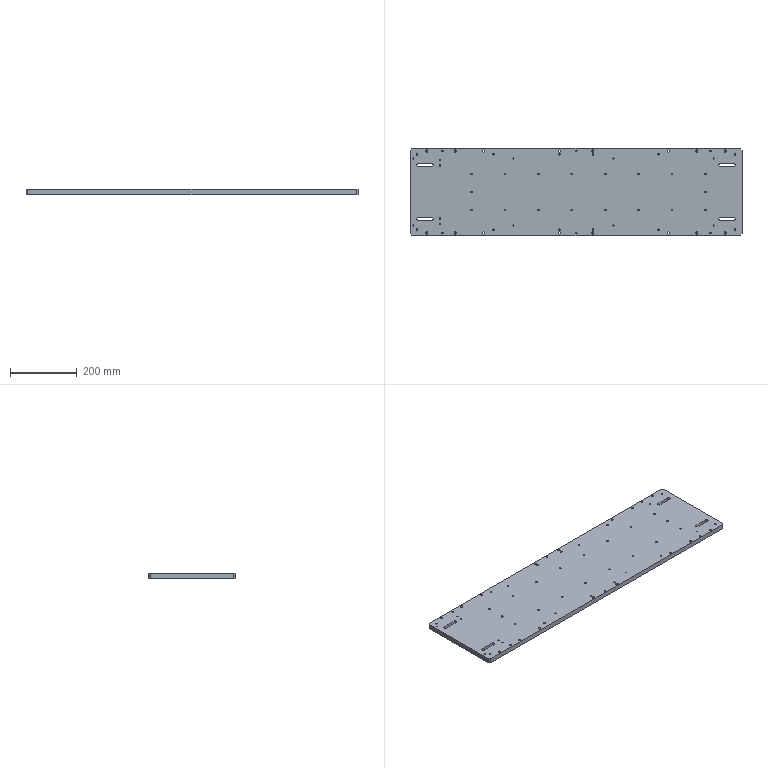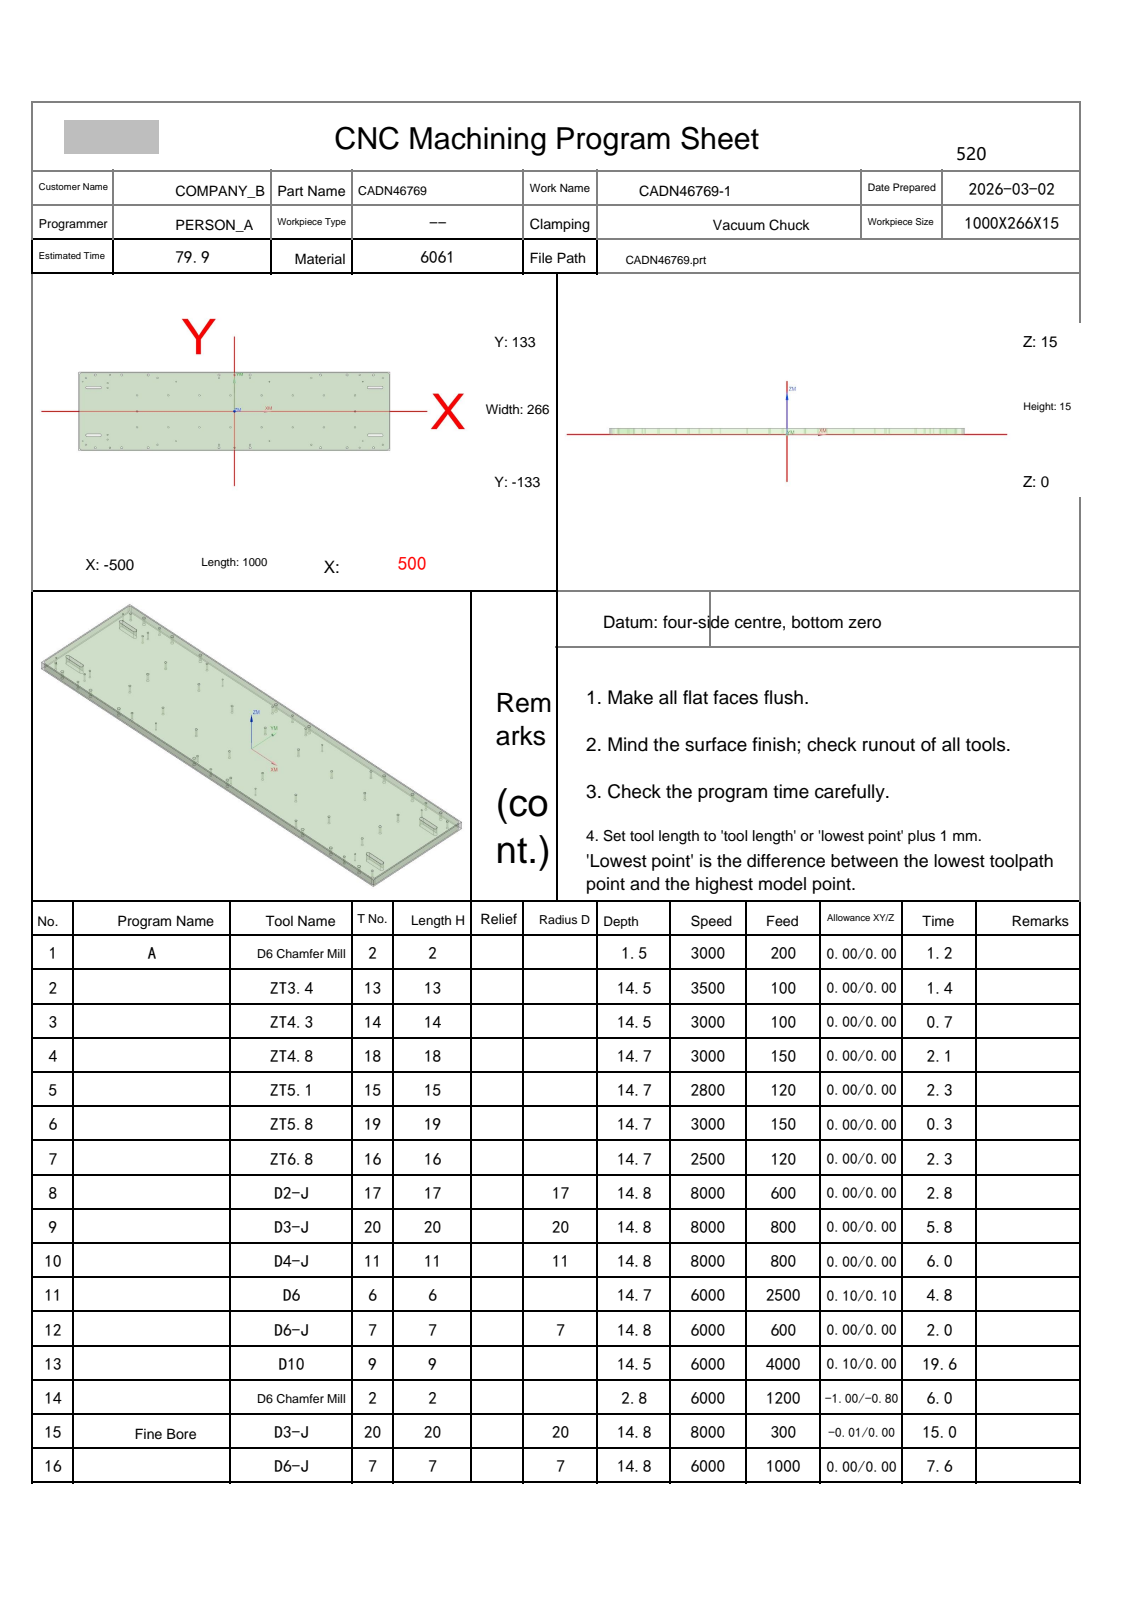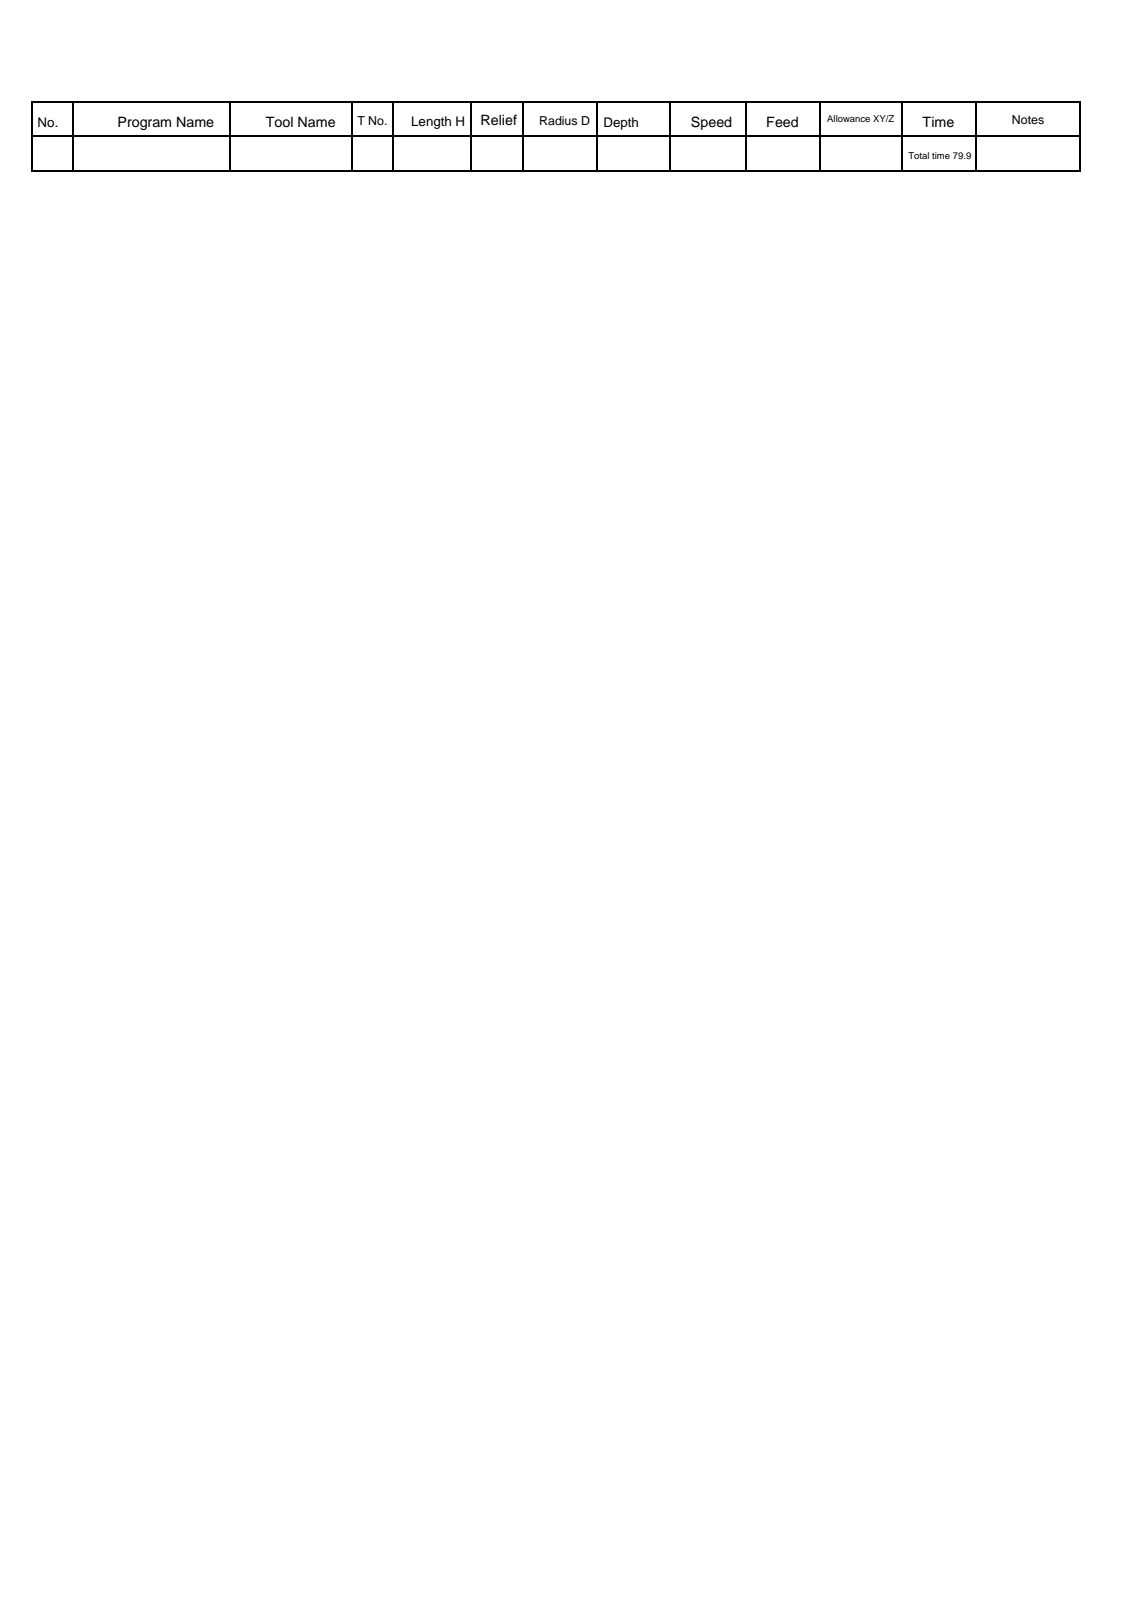NC program | NX | posted by the shop | part box 995 x 261 x 15 mm
Lines 235 to 1015 of 14350:
N8 T17 M06
(D2-J  D=2. R=0. H=17 ce=0.00 di=0.00)
G00 G90 G54 X-486.9 Y-100.369 M03 S8000
G43 H17 Z45.
M08
Z15.5
G01 X-486.943 Y-100.227 Z15.492 F600.
X-487.061 Y-100.061 Z15.482
X-487.227 Y-99.943 Z15.471
X-487.421 Y-99.884 Z15.46
X-487.579 Z15.452
X-487.765 Y-99.939 Z15.442
X-487.926 Y-100.049 Z15.432
X-488.045 Y-100.203 Z15.421
X-488.11 Y-100.386 Z15.411
X-488.116 Y-100.579 Z15.401
X-488.057 Y-100.773 Z15.39
X-487.939 Y-100.939 Z15.38
X-487.773 Y-101.057 Z15.369
X-487.579 Y-101.116 Z15.358
X-487.421 Z15.35
X-487.227 Y-101.057 Z15.34
X-487.061 Y-100.939 Z15.329
X-486.943 Y-100.773 Z15.318
X-486.884 Y-100.579 Z15.308
Y-100.421 Z15.299
X-486.943 Y-100.227 Z15.289
X-487.061 Y-100.061 Z15.278
X-487.227 Y-99.943 Z15.267
X-487.421 Y-99.884 Z15.257
X-487.579 Z15.248
X-487.765 Y-99.939 Z15.238
X-487.926 Y-100.049 Z15.228
X-488.045 Y-100.203 Z15.218
X-488.11 Y-100.386 Z15.208
X-488.116 Y-100.579 Z15.198
X-488.057 Y-100.773 Z15.187
X-487.939 Y-100.939 Z15.176
X-487.773 Y-101.057 Z15.166
X-487.579 Y-101.116 Z15.155
X-487.421 Z15.147
X-487.227 Y-101.057 Z15.136
X-487.061 Y-100.939 Z15.125
X-486.943 Y-100.773 Z15.115
X-486.884 Y-100.579 Z15.104
Y-100.421 Z15.096
X-486.943 Y-100.227 Z15.085
X-487.061 Y-100.061 Z15.074
X-487.227 Y-99.943 Z15.064
X-487.421 Y-99.884 Z15.053
X-487.579 Z15.045
X-487.765 Y-99.939 Z15.035
X-487.926 Y-100.049 Z15.025
X-488.045 Y-100.203 Z15.014
X-488.11 Y-100.386 Z15.004
X-488.115 Y-100.465 Z15.
G41 D17
X-488.15 Y-100.5
G03 X-487.5 Y-101.15 Z14.914 I.65 J0.0
X-486.85 Y-100.5 Z14.828 I0.0 J.65
X-487.5 Y-99.85 Z14.742 I-.65 J0.0
X-488.15 Y-100.5 Z14.656 I0.0 J-.65
X-487.5 Y-101.15 Z14.57 I.65 J0.0
X-486.85 Y-100.5 Z14.484 I0.0 J.65
X-487.5 Y-99.85 Z14.398 I-.65 J0.0
X-488.15 Y-100.5 Z14.312 I0.0 J-.65
X-487.5 Y-101.15 Z14.226 I.65 J0.0
X-486.85 Y-100.5 Z14.14 I0.0 J.65
X-487.5 Y-99.85 Z14.053 I-.65 J0.0
X-488.15 Y-100.5 Z13.967 I0.0 J-.65
X-487.5 Y-101.15 Z13.881 I.65 J0.0
X-486.85 Y-100.5 Z13.795 I0.0 J.65
X-487.5 Y-99.85 Z13.709 I-.65 J0.0
X-488.15 Y-100.5 Z13.623 I0.0 J-.65
X-487.5 Y-101.15 Z13.537 I.65 J0.0
X-486.85 Y-100.5 Z13.451 I0.0 J.65
X-487.5 Y-99.85 Z13.365 I-.65 J0.0
X-488.15 Y-100.5 Z13.279 I0.0 J-.65
X-487.5 Y-101.15 Z13.193 I.65 J0.0
X-486.85 Y-100.5 Z13.107 I0.0 J.65
X-487.5 Y-99.85 Z13.021 I-.65 J0.0
X-488.15 Y-100.5 Z12.935 I0.0 J-.65
X-487.5 Y-101.15 Z12.849 I.65 J0.0
X-486.85 Y-100.5 Z12.763 I0.0 J.65
X-487.5 Y-99.85 Z12.677 I-.65 J0.0
X-488.15 Y-100.5 Z12.591 I0.0 J-.65
X-487.5 Y-101.15 Z12.505 I.65 J0.0
X-486.85 Y-100.5 Z12.419 I0.0 J.65
X-487.5 Y-99.85 Z12.333 I-.65 J0.0
X-488.15 Y-100.5 Z12.247 I0.0 J-.65
X-487.5 Y-101.15 Z12.16 I.65 J0.0
X-486.85 Y-100.5 Z12.074 I0.0 J.65
X-487.5 Y-99.85 Z11.988 I-.65 J0.0
X-488.15 Y-100.5 Z11.902 I0.0 J-.65
X-487.5 Y-101.15 Z11.816 I.65 J0.0
X-486.85 Y-100.5 Z11.73 I0.0 J.65
X-487.5 Y-99.85 Z11.644 I-.65 J0.0
X-488.15 Y-100.5 Z11.558 I0.0 J-.65
X-487.5 Y-101.15 Z11.472 I.65 J0.0
X-486.85 Y-100.5 Z11.386 I0.0 J.65
X-487.5 Y-99.85 Z11.3 I-.65 J0.0
X-488.15 Y-100.5 Z11.214 I0.0 J-.65
X-487.5 Y-101.15 Z11.128 I.65 J0.0
X-486.85 Y-100.5 Z11.042 I0.0 J.65
X-487.5 Y-99.85 Z10.956 I-.65 J0.0
X-488.15 Y-100.5 Z10.87 I0.0 J-.65
X-487.5 Y-101.15 Z10.784 I.65 J0.0
X-486.85 Y-100.5 Z10.698 I0.0 J.65
X-487.5 Y-99.85 Z10.612 I-.65 J0.0
X-488.15 Y-100.5 Z10.526 I0.0 J-.65
X-487.5 Y-101.15 Z10.44 I.65 J0.0
X-486.85 Y-100.5 Z10.353 I0.0 J.65
X-487.5 Y-99.85 Z10.267 I-.65 J0.0
X-488.15 Y-100.5 Z10.181 I0.0 J-.65
X-487.5 Y-101.15 Z10.095 I.65 J0.0
X-486.85 Y-100.5 Z10.009 I0.0 J.65
X-487.5 Y-99.85 Z9.923 I-.65 J0.0
X-488.15 Y-100.5 Z9.837 I0.0 J-.65
X-487.5 Y-101.15 Z9.751 I.65 J0.0
X-486.85 Y-100.5 Z9.665 I0.0 J.65
X-487.5 Y-99.85 Z9.579 I-.65 J0.0
X-488.15 Y-100.5 Z9.493 I0.0 J-.65
X-487.5 Y-101.15 Z9.407 I.65 J0.0
X-486.85 Y-100.5 Z9.321 I0.0 J.65
X-487.5 Y-99.85 Z9.235 I-.65 J0.0
X-488.15 Y-100.5 Z9.149 I0.0 J-.65
X-487.5 Y-101.15 Z9.063 I.65 J0.0
X-486.85 Y-100.5 Z8.977 I0.0 J.65
X-487.5 Y-99.85 Z8.891 I-.65 J0.0
X-488.15 Y-100.5 Z8.805 I0.0 J-.65
X-487.5 Y-101.15 Z8.719 I.65 J0.0
X-486.85 Y-100.5 Z8.633 I0.0 J.65
X-487.5 Y-99.85 Z8.547 I-.65 J0.0
X-488.15 Y-100.5 Z8.46 I0.0 J-.65
X-487.5 Y-101.15 Z8.374 I.65 J0.0
X-486.85 Y-100.5 Z8.288 I0.0 J.65
X-487.5 Y-99.85 Z8.202 I-.65 J0.0
X-488.15 Y-100.5 Z8.116 I0.0 J-.65
X-487.5 Y-101.15 Z8.03 I.65 J0.0
X-486.85 Y-100.5 Z7.944 I0.0 J.65
X-487.5 Y-99.85 Z7.858 I-.65 J0.0
X-488.15 Y-100.5 Z7.772 I0.0 J-.65
X-487.5 Y-101.15 Z7.686 I.65 J0.0
X-486.85 Y-100.5 Z7.6 I0.0 J.65
X-487.5 Y-99.85 Z7.514 I-.65 J0.0
X-488.15 Y-100.5 Z7.428 I0.0 J-.65
X-487.5 Y-101.15 Z7.342 I.65 J0.0
X-486.85 Y-100.5 Z7.256 I0.0 J.65
X-487.5 Y-99.85 Z7.17 I-.65 J0.0
X-488.15 Y-100.5 Z7.084 I0.0 J-.65
X-487.5 Y-101.15 Z6.998 I.65 J0.0
X-486.85 Y-100.5 Z6.912 I0.0 J.65
X-487.5 Y-99.85 Z6.826 I-.65 J0.0
X-488.15 Y-100.5 Z6.74 I0.0 J-.65
X-487.5 Y-101.15 Z6.653 I.65 J0.0
X-486.85 Y-100.5 Z6.567 I0.0 J.65
X-487.5 Y-99.85 Z6.481 I-.65 J0.0
X-488.15 Y-100.5 Z6.395 I0.0 J-.65
X-487.5 Y-101.15 Z6.309 I.65 J0.0
X-486.85 Y-100.5 Z6.223 I0.0 J.65
X-487.5 Y-99.85 Z6.137 I-.65 J0.0
X-488.15 Y-100.5 Z6.051 I0.0 J-.65
X-487.5 Y-101.15 Z5.965 I.65 J0.0
X-486.85 Y-100.5 Z5.879 I0.0 J.65
X-487.5 Y-99.85 Z5.793 I-.65 J0.0
X-488.15 Y-100.5 Z5.707 I0.0 J-.65
X-487.5 Y-101.15 Z5.621 I.65 J0.0
X-486.85 Y-100.5 Z5.535 I0.0 J.65
X-487.5 Y-99.85 Z5.449 I-.65 J0.0
X-488.15 Y-100.5 Z5.363 I0.0 J-.65
X-487.5 Y-101.15 Z5.277 I.65 J0.0
X-486.85 Y-100.5 Z5.191 I0.0 J.65
X-487.5 Y-99.85 Z5.105 I-.65 J0.0
X-488.15 Y-100.5 Z5.019 I0.0 J-.65
X-487.5 Y-101.15 Z4.933 I.65 J0.0
X-486.85 Y-100.5 Z4.847 I0.0 J.65
X-487.5 Y-99.85 Z4.76 I-.65 J0.0
X-488.15 Y-100.5 Z4.674 I0.0 J-.65
X-487.5 Y-101.15 Z4.588 I.65 J0.0
X-486.85 Y-100.5 Z4.502 I0.0 J.65
X-487.5 Y-99.85 Z4.416 I-.65 J0.0
X-488.15 Y-100.5 Z4.33 I0.0 J-.65
X-487.5 Y-101.15 Z4.244 I.65 J0.0
X-486.85 Y-100.5 Z4.158 I0.0 J.65
X-487.5 Y-99.85 Z4.072 I-.65 J0.0
X-488.15 Y-100.5 Z3.986 I0.0 J-.65
X-487.5 Y-101.15 Z3.9 I.65 J0.0
X-486.85 Y-100.5 Z3.814 I0.0 J.65
X-487.5 Y-99.85 Z3.728 I-.65 J0.0
X-488.15 Y-100.5 Z3.642 I0.0 J-.65
X-487.5 Y-101.15 Z3.556 I.65 J0.0
X-486.85 Y-100.5 Z3.47 I0.0 J.65
X-487.5 Y-99.85 Z3.384 I-.65 J0.0
X-488.15 Y-100.5 Z3.298 I0.0 J-.65
X-487.5 Y-101.15 Z3.212 I.65 J0.0
X-486.85 Y-100.5 Z3.126 I0.0 J.65
X-487.5 Y-99.85 Z3.04 I-.65 J0.0
X-488.15 Y-100.5 Z2.953 I0.0 J-.65
X-487.5 Y-101.15 Z2.867 I.65 J0.0
X-486.85 Y-100.5 Z2.781 I0.0 J.65
X-487.5 Y-99.85 Z2.695 I-.65 J0.0
X-488.15 Y-100.5 Z2.609 I0.0 J-.65
X-487.5 Y-101.15 Z2.523 I.65 J0.0
X-486.85 Y-100.5 Z2.437 I0.0 J.65
X-487.5 Y-99.85 Z2.351 I-.65 J0.0
X-488.15 Y-100.5 Z2.265 I0.0 J-.65
X-487.5 Y-101.15 Z2.179 I.65 J0.0
X-486.85 Y-100.5 Z2.093 I0.0 J.65
X-487.5 Y-99.85 Z2.007 I-.65 J0.0
X-488.15 Y-100.5 Z1.921 I0.0 J-.65
X-487.5 Y-101.15 Z1.835 I.65 J0.0
X-486.85 Y-100.5 Z1.749 I0.0 J.65
X-487.5 Y-99.85 Z1.663 I-.65 J0.0
X-488.15 Y-100.5 Z1.577 I0.0 J-.65
X-487.5 Y-101.15 Z1.491 I.65 J0.0
X-486.85 Y-100.5 Z1.405 I0.0 J.65
X-487.5 Y-99.85 Z1.319 I-.65 J0.0
X-488.15 Y-100.5 Z1.233 I0.0 J-.65
X-487.5 Y-101.15 Z1.147 I.65 J0.0
X-486.85 Y-100.5 Z1.06 I0.0 J.65
X-487.5 Y-99.85 Z.974 I-.65 J0.0
X-488.15 Y-100.5 Z.888 I0.0 J-.65
X-487.5 Y-101.15 Z.802 I.65 J0.0
X-486.85 Y-100.5 Z.716 I0.0 J.65
X-487.5 Y-99.85 Z.63 I-.65 J0.0
X-488.15 Y-100.5 Z.544 I0.0 J-.65
X-487.5 Y-101.15 Z.458 I.65 J0.0
X-486.85 Y-100.5 Z.372 I0.0 J.65
X-487.5 Y-99.85 Z.286 I-.65 J0.0
X-488.15 Y-100.5 Z.2 I0.0 J-.65
X-487.5 Y-101.15 I.65 J0.0
X-486.85 Y-100.5 I0.0 J.65
X-487.5 Y-99.85 I-.65 J0.0
X-488.15 Y-100.5 I0.0 J-.65
X-488.031 Y-100.875 I.65 J0.0
G01 X-488.013 Y-100.896
X-487.985 Y-100.901
X-487.961 Y-100.887
G40 X-487.92 Y-100.858
Z1.2
G00 Z45.
X-486.9 Y100.631
Z15.5
G01 X-486.943 Y100.773 Z15.492
X-487.061 Y100.939 Z15.482
X-487.227 Y101.057 Z15.471
X-487.421 Y101.116 Z15.46
X-487.579 Z15.452
X-487.765 Y101.061 Z15.442
X-487.926 Y100.951 Z15.432
X-488.045 Y100.797 Z15.421
X-488.11 Y100.614 Z15.411
X-488.116 Y100.421 Z15.401
X-488.057 Y100.227 Z15.39
X-487.939 Y100.061 Z15.38
X-487.773 Y99.943 Z15.369
X-487.579 Y99.884 Z15.358
X-487.421 Z15.35
X-487.227 Y99.943 Z15.34
X-487.061 Y100.061 Z15.329
X-486.943 Y100.227 Z15.318
X-486.884 Y100.421 Z15.308
Y100.579 Z15.299
X-486.943 Y100.773 Z15.289
X-487.061 Y100.939 Z15.278
X-487.227 Y101.057 Z15.267
X-487.421 Y101.116 Z15.257
X-487.579 Z15.248
X-487.765 Y101.061 Z15.238
X-487.926 Y100.951 Z15.228
X-488.045 Y100.797 Z15.218
X-488.11 Y100.614 Z15.208
X-488.116 Y100.421 Z15.198
X-488.057 Y100.227 Z15.187
X-487.939 Y100.061 Z15.176
X-487.773 Y99.943 Z15.166
X-487.579 Y99.884 Z15.155
X-487.421 Z15.147
X-487.227 Y99.943 Z15.136
X-487.061 Y100.061 Z15.125
X-486.943 Y100.227 Z15.115
X-486.884 Y100.421 Z15.104
Y100.579 Z15.096
X-486.943 Y100.773 Z15.085
X-487.061 Y100.939 Z15.074
X-487.227 Y101.057 Z15.064
X-487.421 Y101.116 Z15.053
X-487.579 Z15.045
X-487.765 Y101.061 Z15.035
X-487.926 Y100.951 Z15.025
X-488.045 Y100.797 Z15.014
X-488.11 Y100.614 Z15.004
X-488.115 Y100.535 Z15.
G41 D17
X-488.15 Y100.5
G03 X-487.5 Y99.85 Z14.914 I.65 J0.0
X-486.85 Y100.5 Z14.828 I0.0 J.65
X-487.5 Y101.15 Z14.742 I-.65 J0.0
X-488.15 Y100.5 Z14.656 I0.0 J-.65
X-487.5 Y99.85 Z14.57 I.65 J0.0
X-486.85 Y100.5 Z14.484 I0.0 J.65
X-487.5 Y101.15 Z14.398 I-.65 J0.0
X-488.15 Y100.5 Z14.312 I0.0 J-.65
X-487.5 Y99.85 Z14.226 I.65 J0.0
X-486.85 Y100.5 Z14.14 I0.0 J.65
X-487.5 Y101.15 Z14.053 I-.65 J0.0
X-488.15 Y100.5 Z13.967 I0.0 J-.65
X-487.5 Y99.85 Z13.881 I.65 J0.0
X-486.85 Y100.5 Z13.795 I0.0 J.65
X-487.5 Y101.15 Z13.709 I-.65 J0.0
X-488.15 Y100.5 Z13.623 I0.0 J-.65
X-487.5 Y99.85 Z13.537 I.65 J0.0
X-486.85 Y100.5 Z13.451 I0.0 J.65
X-487.5 Y101.15 Z13.365 I-.65 J0.0
X-488.15 Y100.5 Z13.279 I0.0 J-.65
X-487.5 Y99.85 Z13.193 I.65 J0.0
X-486.85 Y100.5 Z13.107 I0.0 J.65
X-487.5 Y101.15 Z13.021 I-.65 J0.0
X-488.15 Y100.5 Z12.935 I0.0 J-.65
X-487.5 Y99.85 Z12.849 I.65 J0.0
X-486.85 Y100.5 Z12.763 I0.0 J.65
X-487.5 Y101.15 Z12.677 I-.65 J0.0
X-488.15 Y100.5 Z12.591 I0.0 J-.65
X-487.5 Y99.85 Z12.505 I.65 J0.0
X-486.85 Y100.5 Z12.419 I0.0 J.65
X-487.5 Y101.15 Z12.333 I-.65 J0.0
X-488.15 Y100.5 Z12.247 I0.0 J-.65
X-487.5 Y99.85 Z12.16 I.65 J0.0
X-486.85 Y100.5 Z12.074 I0.0 J.65
X-487.5 Y101.15 Z11.988 I-.65 J0.0
X-488.15 Y100.5 Z11.902 I0.0 J-.65
X-487.5 Y99.85 Z11.816 I.65 J0.0
X-486.85 Y100.5 Z11.73 I0.0 J.65
X-487.5 Y101.15 Z11.644 I-.65 J0.0
X-488.15 Y100.5 Z11.558 I0.0 J-.65
X-487.5 Y99.85 Z11.472 I.65 J0.0
X-486.85 Y100.5 Z11.386 I0.0 J.65
X-487.5 Y101.15 Z11.3 I-.65 J0.0
X-488.15 Y100.5 Z11.214 I0.0 J-.65
X-487.5 Y99.85 Z11.128 I.65 J0.0
X-486.85 Y100.5 Z11.042 I0.0 J.65
X-487.5 Y101.15 Z10.956 I-.65 J0.0
X-488.15 Y100.5 Z10.87 I0.0 J-.65
X-487.5 Y99.85 Z10.784 I.65 J0.0
X-486.85 Y100.5 Z10.698 I0.0 J.65
X-487.5 Y101.15 Z10.612 I-.65 J0.0
X-488.15 Y100.5 Z10.526 I0.0 J-.65
X-487.5 Y99.85 Z10.44 I.65 J0.0
X-486.85 Y100.5 Z10.353 I0.0 J.65
X-487.5 Y101.15 Z10.267 I-.65 J0.0
X-488.15 Y100.5 Z10.181 I0.0 J-.65
X-487.5 Y99.85 Z10.095 I.65 J0.0
X-486.85 Y100.5 Z10.009 I0.0 J.65
X-487.5 Y101.15 Z9.923 I-.65 J0.0
X-488.15 Y100.5 Z9.837 I0.0 J-.65
X-487.5 Y99.85 Z9.751 I.65 J0.0
X-486.85 Y100.5 Z9.665 I0.0 J.65
X-487.5 Y101.15 Z9.579 I-.65 J0.0
X-488.15 Y100.5 Z9.493 I0.0 J-.65
X-487.5 Y99.85 Z9.407 I.65 J0.0
X-486.85 Y100.5 Z9.321 I0.0 J.65
X-487.5 Y101.15 Z9.235 I-.65 J0.0
X-488.15 Y100.5 Z9.149 I0.0 J-.65
X-487.5 Y99.85 Z9.063 I.65 J0.0
X-486.85 Y100.5 Z8.977 I0.0 J.65
X-487.5 Y101.15 Z8.891 I-.65 J0.0
X-488.15 Y100.5 Z8.805 I0.0 J-.65
X-487.5 Y99.85 Z8.719 I.65 J0.0
X-486.85 Y100.5 Z8.633 I0.0 J.65
X-487.5 Y101.15 Z8.547 I-.65 J0.0
X-488.15 Y100.5 Z8.46 I0.0 J-.65
X-487.5 Y99.85 Z8.374 I.65 J0.0
X-486.85 Y100.5 Z8.288 I0.0 J.65
X-487.5 Y101.15 Z8.202 I-.65 J0.0
X-488.15 Y100.5 Z8.116 I0.0 J-.65
X-487.5 Y99.85 Z8.03 I.65 J0.0
X-486.85 Y100.5 Z7.944 I0.0 J.65
X-487.5 Y101.15 Z7.858 I-.65 J0.0
X-488.15 Y100.5 Z7.772 I0.0 J-.65
X-487.5 Y99.85 Z7.686 I.65 J0.0
X-486.85 Y100.5 Z7.6 I0.0 J.65
X-487.5 Y101.15 Z7.514 I-.65 J0.0
X-488.15 Y100.5 Z7.428 I0.0 J-.65
X-487.5 Y99.85 Z7.342 I.65 J0.0
X-486.85 Y100.5 Z7.256 I0.0 J.65
X-487.5 Y101.15 Z7.17 I-.65 J0.0
X-488.15 Y100.5 Z7.084 I0.0 J-.65
X-487.5 Y99.85 Z6.998 I.65 J0.0
X-486.85 Y100.5 Z6.912 I0.0 J.65
X-487.5 Y101.15 Z6.826 I-.65 J0.0
X-488.15 Y100.5 Z6.74 I0.0 J-.65
X-487.5 Y99.85 Z6.653 I.65 J0.0
X-486.85 Y100.5 Z6.567 I0.0 J.65
X-487.5 Y101.15 Z6.481 I-.65 J0.0
X-488.15 Y100.5 Z6.395 I0.0 J-.65
X-487.5 Y99.85 Z6.309 I.65 J0.0
X-486.85 Y100.5 Z6.223 I0.0 J.65
X-487.5 Y101.15 Z6.137 I-.65 J0.0
X-488.15 Y100.5 Z6.051 I0.0 J-.65
X-487.5 Y99.85 Z5.965 I.65 J0.0
X-486.85 Y100.5 Z5.879 I0.0 J.65
X-487.5 Y101.15 Z5.793 I-.65 J0.0
X-488.15 Y100.5 Z5.707 I0.0 J-.65
X-487.5 Y99.85 Z5.621 I.65 J0.0
X-486.85 Y100.5 Z5.535 I0.0 J.65
X-487.5 Y101.15 Z5.449 I-.65 J0.0
X-488.15 Y100.5 Z5.363 I0.0 J-.65
X-487.5 Y99.85 Z5.277 I.65 J0.0
X-486.85 Y100.5 Z5.191 I0.0 J.65
X-487.5 Y101.15 Z5.105 I-.65 J0.0
X-488.15 Y100.5 Z5.019 I0.0 J-.65
X-487.5 Y99.85 Z4.933 I.65 J0.0
X-486.85 Y100.5 Z4.847 I0.0 J.65
X-487.5 Y101.15 Z4.76 I-.65 J0.0
X-488.15 Y100.5 Z4.674 I0.0 J-.65
X-487.5 Y99.85 Z4.588 I.65 J0.0
X-486.85 Y100.5 Z4.502 I0.0 J.65
X-487.5 Y101.15 Z4.416 I-.65 J0.0
X-488.15 Y100.5 Z4.33 I0.0 J-.65
X-487.5 Y99.85 Z4.244 I.65 J0.0
X-486.85 Y100.5 Z4.158 I0.0 J.65
X-487.5 Y101.15 Z4.072 I-.65 J0.0
X-488.15 Y100.5 Z3.986 I0.0 J-.65
X-487.5 Y99.85 Z3.9 I.65 J0.0
X-486.85 Y100.5 Z3.814 I0.0 J.65
X-487.5 Y101.15 Z3.728 I-.65 J0.0
X-488.15 Y100.5 Z3.642 I0.0 J-.65
X-487.5 Y99.85 Z3.556 I.65 J0.0
X-486.85 Y100.5 Z3.47 I0.0 J.65
X-487.5 Y101.15 Z3.384 I-.65 J0.0
X-488.15 Y100.5 Z3.298 I0.0 J-.65
X-487.5 Y99.85 Z3.212 I.65 J0.0
X-486.85 Y100.5 Z3.126 I0.0 J.65
X-487.5 Y101.15 Z3.04 I-.65 J0.0
X-488.15 Y100.5 Z2.953 I0.0 J-.65
X-487.5 Y99.85 Z2.867 I.65 J0.0
X-486.85 Y100.5 Z2.781 I0.0 J.65
X-487.5 Y101.15 Z2.695 I-.65 J0.0
X-488.15 Y100.5 Z2.609 I0.0 J-.65
X-487.5 Y99.85 Z2.523 I.65 J0.0
X-486.85 Y100.5 Z2.437 I0.0 J.65
X-487.5 Y101.15 Z2.351 I-.65 J0.0
X-488.15 Y100.5 Z2.265 I0.0 J-.65
X-487.5 Y99.85 Z2.179 I.65 J0.0
X-486.85 Y100.5 Z2.093 I0.0 J.65
X-487.5 Y101.15 Z2.007 I-.65 J0.0
X-488.15 Y100.5 Z1.921 I0.0 J-.65
X-487.5 Y99.85 Z1.835 I.65 J0.0
X-486.85 Y100.5 Z1.749 I0.0 J.65
X-487.5 Y101.15 Z1.663 I-.65 J0.0
X-488.15 Y100.5 Z1.577 I0.0 J-.65
X-487.5 Y99.85 Z1.491 I.65 J0.0
X-486.85 Y100.5 Z1.405 I0.0 J.65
X-487.5 Y101.15 Z1.319 I-.65 J0.0
X-488.15 Y100.5 Z1.233 I0.0 J-.65
X-487.5 Y99.85 Z1.147 I.65 J0.0
X-486.85 Y100.5 Z1.06 I0.0 J.65
X-487.5 Y101.15 Z.974 I-.65 J0.0
X-488.15 Y100.5 Z.888 I0.0 J-.65
X-487.5 Y99.85 Z.802 I.65 J0.0
X-486.85 Y100.5 Z.716 I0.0 J.65
X-487.5 Y101.15 Z.63 I-.65 J0.0
X-488.15 Y100.5 Z.544 I0.0 J-.65
X-487.5 Y99.85 Z.458 I.65 J0.0
X-486.85 Y100.5 Z.372 I0.0 J.65
X-487.5 Y101.15 Z.286 I-.65 J0.0
X-488.15 Y100.5 Z.2 I0.0 J-.65
X-487.5 Y99.85 I.65 J0.0
X-486.85 Y100.5 I0.0 J.65
X-487.5 Y101.15 I-.65 J0.0
X-488.15 Y100.5 I0.0 J-.65
X-488.031 Y100.125 I.65 J0.0
G01 X-488.013 Y100.104
X-487.985 Y100.099
X-487.961 Y100.113
G40 X-487.92 Y100.142
Z1.2
G00 Z45.
X-187.369 Y99.9
Z15.5
G01 X-187.227 Y99.943 Z15.492
X-187.061 Y100.061 Z15.482
X-186.943 Y100.227 Z15.471
X-186.884 Y100.421 Z15.46
Y100.579 Z15.452
X-186.939 Y100.765 Z15.442
X-187.049 Y100.926 Z15.432
X-187.203 Y101.045 Z15.421
X-187.386 Y101.11 Z15.411
X-187.579 Y101.116 Z15.401
X-187.773 Y101.057 Z15.39
X-187.939 Y100.939 Z15.38
X-188.057 Y100.773 Z15.369
X-188.116 Y100.579 Z15.358
Y100.421 Z15.35
X-188.057 Y100.227 Z15.34
X-187.939 Y100.061 Z15.329
X-187.773 Y99.943 Z15.318
X-187.579 Y99.884 Z15.308
X-187.421 Z15.299
X-187.227 Y99.943 Z15.289
X-187.061 Y100.061 Z15.278
X-186.943 Y100.227 Z15.267
X-186.884 Y100.421 Z15.257
Y100.579 Z15.248
X-186.939 Y100.765 Z15.238
X-187.049 Y100.926 Z15.228
X-187.203 Y101.045 Z15.218
X-187.386 Y101.11 Z15.208
X-187.579 Y101.116 Z15.198
X-187.773 Y101.057 Z15.187
X-187.939 Y100.939 Z15.176
X-188.057 Y100.773 Z15.166
X-188.116 Y100.579 Z15.155
Y100.421 Z15.147
X-188.057 Y100.227 Z15.136
X-187.939 Y100.061 Z15.125
X-187.773 Y99.943 Z15.115
X-187.579 Y99.884 Z15.104
X-187.421 Z15.096
X-187.227 Y99.943 Z15.085
X-187.061 Y100.061 Z15.074
X-186.943 Y100.227 Z15.064
X-186.884 Y100.421 Z15.053
Y100.579 Z15.045
X-186.939 Y100.765 Z15.035
X-187.049 Y100.926 Z15.025
X-187.203 Y101.045 Z15.014
X-187.386 Y101.11 Z15.004
X-187.465 Y101.115 Z15.
G41 D17
X-187.5 Y101.15
G03 X-188.15 Y100.5 Z14.914 I0.0 J-.65
X-187.5 Y99.85 Z14.828 I.65 J0.0
X-186.85 Y100.5 Z14.742 I0.0 J.65
X-187.5 Y101.15 Z14.656 I-.65 J0.0
X-188.15 Y100.5 Z14.57 I0.0 J-.65
X-187.5 Y99.85 Z14.484 I.65 J0.0
X-186.85 Y100.5 Z14.398 I0.0 J.65
X-187.5 Y101.15 Z14.312 I-.65 J0.0
X-188.15 Y100.5 Z14.226 I0.0 J-.65
X-187.5 Y99.85 Z14.14 I.65 J0.0
X-186.85 Y100.5 Z14.053 I0.0 J.65
X-187.5 Y101.15 Z13.967 I-.65 J0.0
X-188.15 Y100.5 Z13.881 I0.0 J-.65
X-187.5 Y99.85 Z13.795 I.65 J0.0
X-186.85 Y100.5 Z13.709 I0.0 J.65
X-187.5 Y101.15 Z13.623 I-.65 J0.0
X-188.15 Y100.5 Z13.537 I0.0 J-.65
X-187.5 Y99.85 Z13.451 I.65 J0.0
X-186.85 Y100.5 Z13.365 I0.0 J.65
X-187.5 Y101.15 Z13.279 I-.65 J0.0
X-188.15 Y100.5 Z13.193 I0.0 J-.65
X-187.5 Y99.85 Z13.107 I.65 J0.0
X-186.85 Y100.5 Z13.021 I0.0 J.65
X-187.5 Y101.15 Z12.935 I-.65 J0.0
X-188.15 Y100.5 Z12.849 I0.0 J-.65
X-187.5 Y99.85 Z12.763 I.65 J0.0
X-186.85 Y100.5 Z12.677 I0.0 J.65
X-187.5 Y101.15 Z12.591 I-.65 J0.0
X-188.15 Y100.5 Z12.505 I0.0 J-.65
X-187.5 Y99.85 Z12.419 I.65 J0.0
X-186.85 Y100.5 Z12.333 I0.0 J.65
X-187.5 Y101.15 Z12.247 I-.65 J0.0
X-188.15 Y100.5 Z12.16 I0.0 J-.65
X-187.5 Y99.85 Z12.074 I.65 J0.0
X-186.85 Y100.5 Z11.988 I0.0 J.65
X-187.5 Y101.15 Z11.902 I-.65 J0.0
X-188.15 Y100.5 Z11.816 I0.0 J-.65
X-187.5 Y99.85 Z11.73 I.65 J0.0
X-186.85 Y100.5 Z11.644 I0.0 J.65
X-187.5 Y101.15 Z11.558 I-.65 J0.0
X-188.15 Y100.5 Z11.472 I0.0 J-.65
X-187.5 Y99.85 Z11.386 I.65 J0.0
X-186.85 Y100.5 Z11.3 I0.0 J.65
X-187.5 Y101.15 Z11.214 I-.65 J0.0
X-188.15 Y100.5 Z11.128 I0.0 J-.65
X-187.5 Y99.85 Z11.042 I.65 J0.0
X-186.85 Y100.5 Z10.956 I0.0 J.65
X-187.5 Y101.15 Z10.87 I-.65 J0.0
X-188.15 Y100.5 Z10.784 I0.0 J-.65
X-187.5 Y99.85 Z10.698 I.65 J0.0
X-186.85 Y100.5 Z10.612 I0.0 J.65
X-187.5 Y101.15 Z10.526 I-.65 J0.0
X-188.15 Y100.5 Z10.44 I0.0 J-.65
X-187.5 Y99.85 Z10.353 I.65 J0.0
X-186.85 Y100.5 Z10.267 I0.0 J.65
X-187.5 Y101.15 Z10.181 I-.65 J0.0
X-188.15 Y100.5 Z10.095 I0.0 J-.65
X-187.5 Y99.85 Z10.009 I.65 J0.0
X-186.85 Y100.5 Z9.923 I0.0 J.65
X-187.5 Y101.15 Z9.837 I-.65 J0.0
X-188.15 Y100.5 Z9.751 I0.0 J-.65
X-187.5 Y99.85 Z9.665 I.65 J0.0
X-186.85 Y100.5 Z9.579 I0.0 J.65
X-187.5 Y101.15 Z9.493 I-.65 J0.0
X-188.15 Y100.5 Z9.407 I0.0 J-.65
X-187.5 Y99.85 Z9.321 I.65 J0.0
X-186.85 Y100.5 Z9.235 I0.0 J.65
X-187.5 Y101.15 Z9.149 I-.65 J0.0
X-188.15 Y100.5 Z9.063 I0.0 J-.65
X-187.5 Y99.85 Z8.977 I.65 J0.0
X-186.85 Y100.5 Z8.891 I0.0 J.65
X-187.5 Y101.15 Z8.805 I-.65 J0.0
X-188.15 Y100.5 Z8.719 I0.0 J-.65
X-187.5 Y99.85 Z8.633 I.65 J0.0
X-186.85 Y100.5 Z8.547 I0.0 J.65
X-187.5 Y101.15 Z8.46 I-.65 J0.0
X-188.15 Y100.5 Z8.374 I0.0 J-.65
X-187.5 Y99.85 Z8.288 I.65 J0.0
X-186.85 Y100.5 Z8.202 I0.0 J.65
X-187.5 Y101.15 Z8.116 I-.65 J0.0
X-188.15 Y100.5 Z8.03 I0.0 J-.65
X-187.5 Y99.85 Z7.944 I.65 J0.0
X-186.85 Y100.5 Z7.858 I0.0 J.65
X-187.5 Y101.15 Z7.772 I-.65 J0.0
X-188.15 Y100.5 Z7.686 I0.0 J-.65
X-187.5 Y99.85 Z7.6 I.65 J0.0
X-186.85 Y100.5 Z7.514 I0.0 J.65
X-187.5 Y101.15 Z7.428 I-.65 J0.0
X-188.15 Y100.5 Z7.342 I0.0 J-.65
X-187.5 Y99.85 Z7.256 I.65 J0.0
X-186.85 Y100.5 Z7.17 I0.0 J.65
X-187.5 Y101.15 Z7.084 I-.65 J0.0
X-188.15 Y100.5 Z6.998 I0.0 J-.65
X-187.5 Y99.85 Z6.912 I.65 J0.0
X-186.85 Y100.5 Z6.826 I0.0 J.65
X-187.5 Y101.15 Z6.74 I-.65 J0.0
X-188.15 Y100.5 Z6.653 I0.0 J-.65
X-187.5 Y99.85 Z6.567 I.65 J0.0
X-186.85 Y100.5 Z6.481 I0.0 J.65
X-187.5 Y101.15 Z6.395 I-.65 J0.0
X-188.15 Y100.5 Z6.309 I0.0 J-.65
X-187.5 Y99.85 Z6.223 I.65 J0.0
X-186.85 Y100.5 Z6.137 I0.0 J.65
X-187.5 Y101.15 Z6.051 I-.65 J0.0
X-188.15 Y100.5 Z5.965 I0.0 J-.65
X-187.5 Y99.85 Z5.879 I.65 J0.0
X-186.85 Y100.5 Z5.793 I0.0 J.65
X-187.5 Y101.15 Z5.707 I-.65 J0.0
X-188.15 Y100.5 Z5.621 I0.0 J-.65
X-187.5 Y99.85 Z5.535 I.65 J0.0
X-186.85 Y100.5 Z5.449 I0.0 J.65
X-187.5 Y101.15 Z5.363 I-.65 J0.0
X-188.15 Y100.5 Z5.277 I0.0 J-.65
X-187.5 Y99.85 Z5.191 I.65 J0.0
X-186.85 Y100.5 Z5.105 I0.0 J.65
X-187.5 Y101.15 Z5.019 I-.65 J0.0
X-188.15 Y100.5 Z4.933 I0.0 J-.65
X-187.5 Y99.85 Z4.847 I.65 J0.0
X-186.85 Y100.5 Z4.76 I0.0 J.65
X-187.5 Y101.15 Z4.674 I-.65 J0.0
X-188.15 Y100.5 Z4.588 I0.0 J-.65
X-187.5 Y99.85 Z4.502 I.65 J0.0
X-186.85 Y100.5 Z4.416 I0.0 J.65
X-187.5 Y101.15 Z4.33 I-.65 J0.0
X-188.15 Y100.5 Z4.244 I0.0 J-.65
X-187.5 Y99.85 Z4.158 I.65 J0.0
X-186.85 Y100.5 Z4.072 I0.0 J.65
X-187.5 Y101.15 Z3.986 I-.65 J0.0
X-188.15 Y100.5 Z3.9 I0.0 J-.65
X-187.5 Y99.85 Z3.814 I.65 J0.0
X-186.85 Y100.5 Z3.728 I0.0 J.65
X-187.5 Y101.15 Z3.642 I-.65 J0.0
X-188.15 Y100.5 Z3.556 I0.0 J-.65
X-187.5 Y99.85 Z3.47 I.65 J0.0
X-186.85 Y100.5 Z3.384 I0.0 J.65
X-187.5 Y101.15 Z3.298 I-.65 J0.0
X-188.15 Y100.5 Z3.212 I0.0 J-.65
X-187.5 Y99.85 Z3.126 I.65 J0.0
X-186.85 Y100.5 Z3.04 I0.0 J.65
X-187.5 Y101.15 Z2.953 I-.65 J0.0
X-188.15 Y100.5 Z2.867 I0.0 J-.65
X-187.5 Y99.85 Z2.781 I.65 J0.0
X-186.85 Y100.5 Z2.695 I0.0 J.65
X-187.5 Y101.15 Z2.609 I-.65 J0.0
X-188.15 Y100.5 Z2.523 I0.0 J-.65
X-187.5 Y99.85 Z2.437 I.65 J0.0
X-186.85 Y100.5 Z2.351 I0.0 J.65
X-187.5 Y101.15 Z2.265 I-.65 J0.0
X-188.15 Y100.5 Z2.179 I0.0 J-.65
X-187.5 Y99.85 Z2.093 I.65 J0.0
X-186.85 Y100.5 Z2.007 I0.0 J.65
X-187.5 Y101.15 Z1.921 I-.65 J0.0
X-188.15 Y100.5 Z1.835 I0.0 J-.65
X-187.5 Y99.85 Z1.749 I.65 J0.0
X-186.85 Y100.5 Z1.663 I0.0 J.65
X-187.5 Y101.15 Z1.577 I-.65 J0.0
X-188.15 Y100.5 Z1.491 I0.0 J-.65
X-187.5 Y99.85 Z1.405 I.65 J0.0
X-186.85 Y100.5 Z1.319 I0.0 J.65
X-187.5 Y101.15 Z1.233 I-.65 J0.0
X-188.15 Y100.5 Z1.147 I0.0 J-.65
X-187.5 Y99.85 Z1.06 I.65 J0.0
X-186.85 Y100.5 Z.974 I0.0 J.65
X-187.5 Y101.15 Z.888 I-.65 J0.0
X-188.15 Y100.5 Z.802 I0.0 J-.65
X-187.5 Y99.85 Z.716 I.65 J0.0
X-186.85 Y100.5 Z.63 I0.0 J.65
X-187.5 Y101.15 Z.544 I-.65 J0.0
X-188.15 Y100.5 Z.458 I0.0 J-.65
X-187.5 Y99.85 Z.372 I.65 J0.0
X-186.85 Y100.5 Z.286 I0.0 J.65
X-187.5 Y101.15 Z.2 I-.65 J0.0
X-188.15 Y100.5 I0.0 J-.65
X-187.5 Y99.85 I.65 J0.0
X-186.85 Y100.5 I0.0 J.65
X-187.5 Y101.15 I-.65 J0.0
X-187.875 Y101.031 I0.0 J-.65
G01 X-187.896 Y101.013
X-187.901 Y100.985
X-187.887 Y100.961
G40 X-187.858 Y100.92
Z1.2
G00 Z45.
X-187.631 Y-99.9
Z15.5
G01 X-187.773 Y-99.943 Z15.492
X-187.939 Y-100.061 Z15.482
X-188.057 Y-100.227 Z15.471
X-188.116 Y-100.421 Z15.46
Y-100.579 Z15.452
X-188.061 Y-100.765 Z15.442
X-187.951 Y-100.926 Z15.432
X-187.797 Y-101.045 Z15.421
X-187.614 Y-101.11 Z15.411
X-187.421 Y-101.116 Z15.401
X-187.227 Y-101.057 Z15.39
X-187.061 Y-100.939 Z15.38
X-186.943 Y-100.773 Z15.369
X-186.884 Y-100.579 Z15.358
Y-100.421 Z15.35
X-186.943 Y-100.227 Z15.34
X-187.061 Y-100.061 Z15.329
X-187.227 Y-99.943 Z15.318
X-187.421 Y-99.884 Z15.308
X-187.579 Z15.299
X-187.773 Y-99.943 Z15.289
X-187.939 Y-100.061 Z15.278
X-188.057 Y-100.227 Z15.267
X-188.116 Y-100.421 Z15.257
Y-100.579 Z15.248
X-188.061 Y-100.765 Z15.238
X-187.951 Y-100.926 Z15.228
X-187.797 Y-101.045 Z15.218
X-187.614 Y-101.11 Z15.208
X-187.421 Y-101.116 Z15.198
X-187.227 Y-101.057 Z15.187
X-187.061 Y-100.939 Z15.176
X-186.943 Y-100.773 Z15.166
X-186.884 Y-100.579 Z15.155
Y-100.421 Z15.147
X-186.943 Y-100.227 Z15.136
X-187.061 Y-100.061 Z15.125
X-187.227 Y-99.943 Z15.115
X-187.421 Y-99.884 Z15.104
X-187.579 Z15.096
X-187.773 Y-99.943 Z15.085
X-187.939 Y-100.061 Z15.074
X-188.057 Y-100.227 Z15.064
X-188.116 Y-100.421 Z15.053
Y-100.579 Z15.045
X-188.061 Y-100.765 Z15.035
X-187.951 Y-100.926 Z15.025
X-187.797 Y-101.045 Z15.014
X-187.614 Y-101.11 Z15.004
X-187.535 Y-101.115 Z15.
G41 D17
X-187.5 Y-101.15
G03 X-186.85 Y-100.5 Z14.914 I0.0 J.65
X-187.5 Y-99.85 Z14.828 I-.65 J0.0
X-188.15 Y-100.5 Z14.742 I0.0 J-.65
X-187.5 Y-101.15 Z14.656 I.65 J0.0
X-186.85 Y-100.5 Z14.57 I0.0 J.65
X-187.5 Y-99.85 Z14.484 I-.65 J0.0
X-188.15 Y-100.5 Z14.398 I0.0 J-.65
X-187.5 Y-101.15 Z14.312 I.65 J0.0
X-186.85 Y-100.5 Z14.226 I0.0 J.65
X-187.5 Y-99.85 Z14.14 I-.65 J0.0
X-188.15 Y-100.5 Z14.053 I0.0 J-.65
X-187.5 Y-101.15 Z13.967 I.65 J0.0